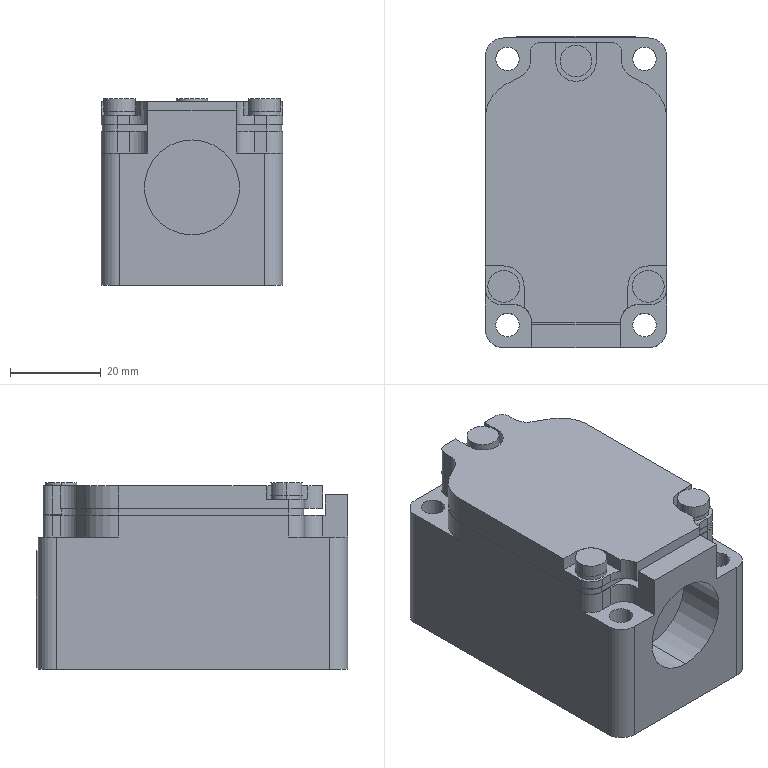Part | SolidWorks | features BaseBody 1 | 1 solid | 152 faces | box 40 x 68.7 x 41.2 mm | volume 97429 mm3 | plane 77 | cylinder 75 | commonest cylinder face diameters 8 x12 7 x10 3.5 x8 5.2 x8 6 x8 6.9 x6